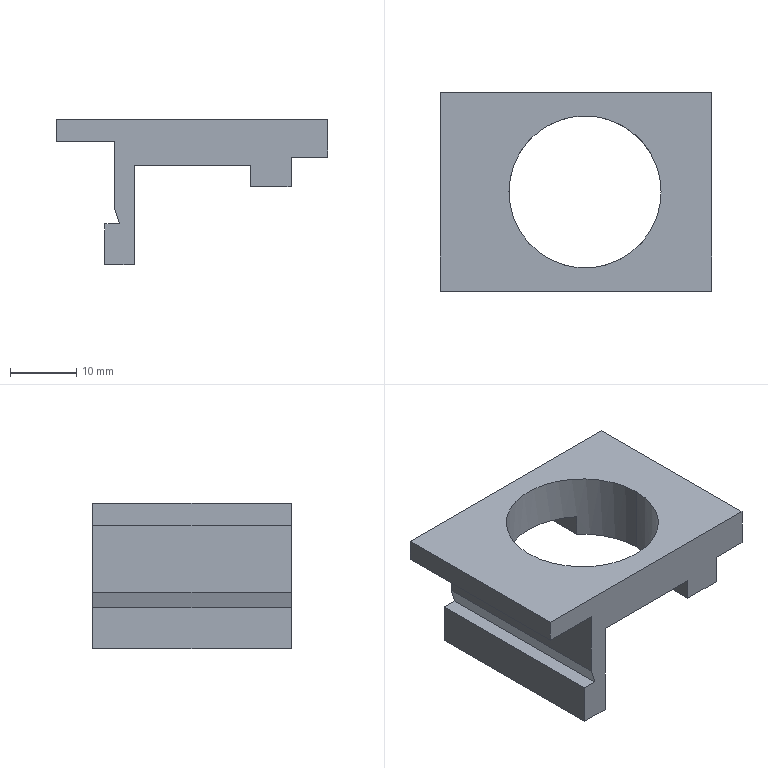Part | STEP file | 1 solid | 22 faces | box 41 x 30 x 22 mm | volume 6377 mm3 | plane 20 | cylinder 2 | commonest cylinder face diameters 23 x2